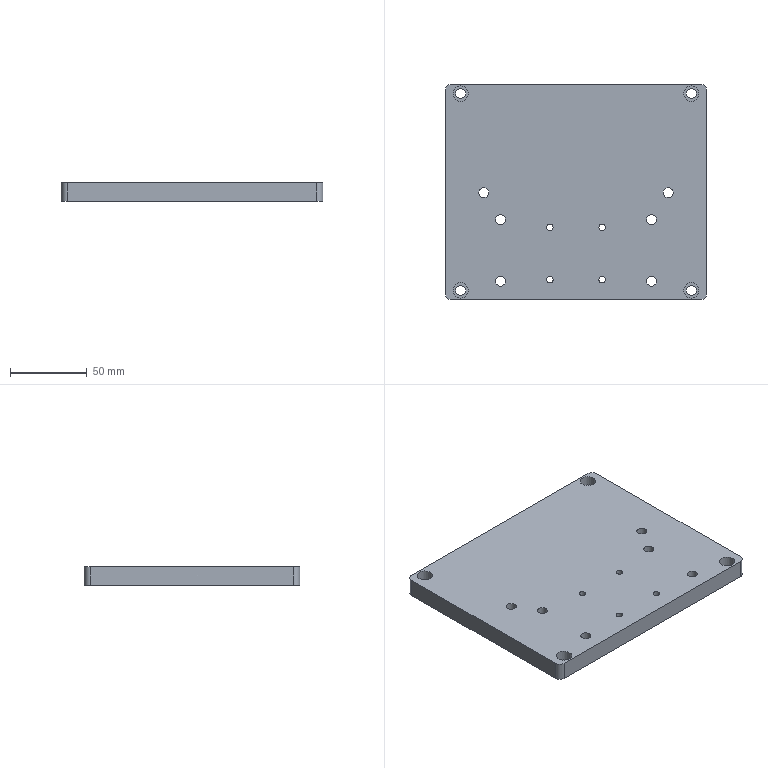Part | STEP file | 1 solid | 44 faces | box 170 x 140 x 12 mm | volume 277366 mm3 | cylinder 28 | plane 16 | commonest cylinder face diameters 6.5 x10 10.5 x6 4.2 x4 8 x4 10 x4